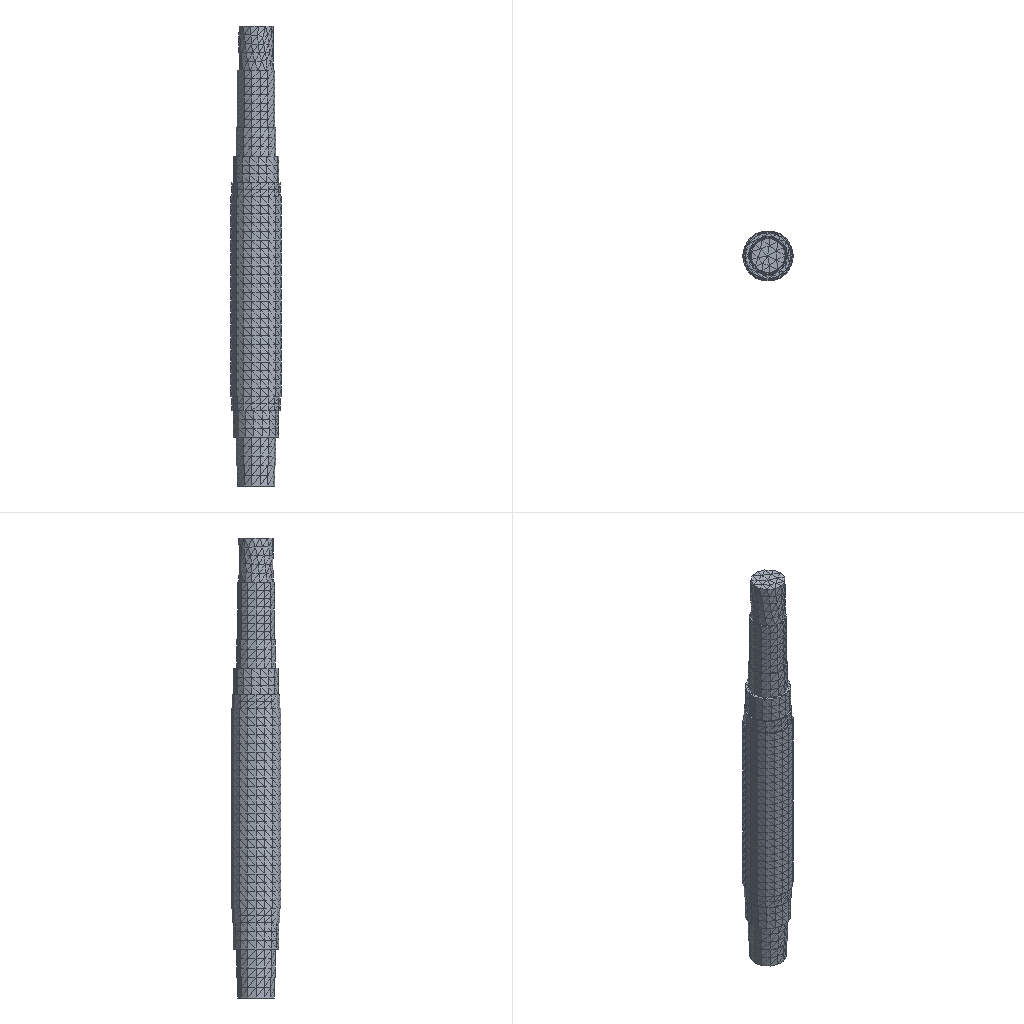Simulation study | abaqus
Set-up summary:
category,name,step,type,value,unit,region
solver,abaqus,,Abaqus/CAE 2024
units,mm-N-s-tonne (MPa),,inferred,E=210000 density=7.89e-09
analysis,Step-1,,static,time_period=1
mesh,nodes,,,14081
mesh,elements,,,8881
element_type,C3D10,,,8881
material,Material-1,,E,210000
material,Material-1,,nu,0.27
material,Material-1,,density,7.89e-09
section,Material-1,,solid section,,,_PickedSet7
load,Load-1,Step-1,concentrated moment,"785000 [dir=(0, 0, 1)]",,_PickedSet15
bc,BC-1,initial,encastre,[dofs=ENCASTRE],,_PickedSet17
constraint,coupling,,,1
Abaqus input file, long lists of numbers shortened:
*Heading
** Job name: deck Model name: Model-1
** Generated by: Abaqus/CAE 2024
*Preprint, echo=NO, model=NO, history=NO, contact=NO
**
** PARTS
**
*Part, name=P1-1
*Node
      1,          16.,          49.,        829.5
      2,         -16.,          49.,        829.5
** (14078 more lines like these left out)
*Element, type=C3D10
   1,  1081,  1082,  1083,  1084,  2064,  2063,  2062,  2066,  2065,  2067
   2,  1081,  1085,  1083,  1086,  2069,  2068,  2062,  2071,  2070,  2072
** (8879 more lines like these left out)
*Nset, nset=_PickedSet7, internal, generate
     1,  14080,      1
*Elset, elset=_PickedSet7, internal, generate
    1,  8881,     1
** Section: Section-1
*Solid Section, elset=_PickedSet7, material=Material-1
,
*End Part
**
**
** ASSEMBLY
**
*Assembly, name=Assembly
**
*Instance, name=P1-1-1, part=P1-1
*End Instance
**
*Node
      1,           0., 3.67394019e-15,         945.
*Nset, nset=_PickedSet12, internal
 1,
*Nset, nset=_PickedSet15, internal
 1,
*Nset, nset=_PickedSet17, internal, instance=P1-1-1
    24,    26,   258,   259,   260,   261,   262,   263,   264,   265,   266,   267,   268,   269,   270,   271
   272,   273,   274,   292,   293,   294,   295,   296,   297,   298,   299,   300,   301,   302,   303,   304
** (10 more lines like these left out)
*Elset, elset=_PickedSet17, internal, instance=P1-1-1
   22,  720,  790, 1405, 1666, 1788, 1795, 1824, 2019, 4998, 5064, 5123, 5139, 5165, 5175, 5198
 5206, 5401, 5412, 5413, 5420, 5431, 5447, 5453, 5458, 5461, 5467, 5470, 5478, 5481, 5497, 5730
** (3 more lines like these left out)
*Elset, elset=__PickedSurf11_S3, internal, instance=P1-1-1
   68,  288,  612,  784, 1630, 1636, 1654, 1665, 1698, 1719, 1731, 1746, 1910, 1927, 1941, 1946
 1947, 1951, 1954, 1959, 1965, 1971, 1972, 1975, 1978, 1983, 1984, 1988, 1993, 1994, 1996, 2004
** (10 more lines like these left out)
*Elset, elset=__PickedSurf11_S1, internal, instance=P1-1-1
 1441, 1740, 1981, 1994, 2010, 2024, 2176, 2183, 2184, 2196, 2224, 2235, 2237, 2242, 2352, 2354
 2405, 2451, 7799, 7981, 8699
*Elset, elset=__PickedSurf11_S4, internal, instance=P1-1-1
 1741, 1991, 2012, 2028, 2155, 2205, 2308, 2349, 2538, 2620, 4460, 5639, 5957, 7536, 8387
*Elset, elset=__PickedSurf11_S2, internal, instance=P1-1-1
 1726, 2006, 2011, 2152, 2176, 2217, 2219, 2233, 2261, 2354, 2417, 2443, 2574, 2580, 2585, 7536
 8855,
*Surface, type=ELEMENT, name=_PickedSurf11, internal
__PickedSurf11_S3, S3
__PickedSurf11_S1, S1
__PickedSurf11_S4, S4
__PickedSurf11_S2, S2
** Constraint: Constraint-1
*Coupling, constraint name=Constraint-1, ref node=_PickedSet12, surface=_PickedSurf11
*Kinematic
*End Assembly
**
** MATERIALS
**
*Material, name=Material-1
*Density
 7.89e-09,
*Elastic
210000., 0.27
**
** BOUNDARY CONDITIONS
**
** Name: BC-1 Type: Symmetry/Antisymmetry/Encastre
*Boundary
_PickedSet17, ENCASTRE
** ----------------------------------------------------------------
**
** STEP: Step-1
**
*Step, name=Step-1, nlgeom=NO, inc=1000
*Static, stabilize=0.0002, allsdtol=0.05, continue=NO
0.1, 1., 1e-05, 0.1
**
** LOADS
**
** Name: Load-1   Type: Moment
*Cload
_PickedSet15, 6, 785000.
**
** OUTPUT REQUESTS
**
*Restart, write, frequency=0
**
** FIELD OUTPUT: F-Output-1
**
*Output, field, variable=PRESELECT
**
** HISTORY OUTPUT: H-Output-1
**
*Output, history, variable=PRESELECT
*End Step
Results summary:
result,odb.job_status,,,JOB_STATUS_COMPLETED_SUCCESSFULLY,"consistent, unstated (Abaqus has no unit system)"
result,steps[0].procedure,Step-1,,*STATIC,"consistent, unstated (Abaqus has no unit system)"
result,steps[0].time_period,Step-1,,1,"consistent, unstated (Abaqus has no unit system)"
result,steps[0].n_frames,Step-1,,11,"consistent, unstated (Abaqus has no unit system)"
result,steps[0].last_frame.id,Step-1,,10,"consistent, unstated (Abaqus has no unit system)"
result,steps[0].last_frame.value,Step-1,,1,"consistent, unstated (Abaqus has no unit system)"
result,steps[0].last_frame.description,Step-1,,Increment     10: Step Time =    1.000,"consistent, unstated (Abaqus has no unit system)"
result,steps[0].completed,Step-1,,True,"consistent, unstated (Abaqus has no unit system)"
result,steps[0].max_U_magnitude,Step-1,,0.007277,"consistent, unstated (Abaqus has no unit system)"
result,steps[0].max_S_mises,Step-1,,7.39,"consistent, unstated (Abaqus has no unit system)"
result,steps[0].RF_sum[1],Step-1,,-0.003649,"consistent, unstated (Abaqus has no unit system)"
result,steps[0].RF_sum[2],Step-1,,-0.001575,"consistent, unstated (Abaqus has no unit system)"
result,steps[0].RF_sum[3],Step-1,,0.0002387,"consistent, unstated (Abaqus has no unit system)"